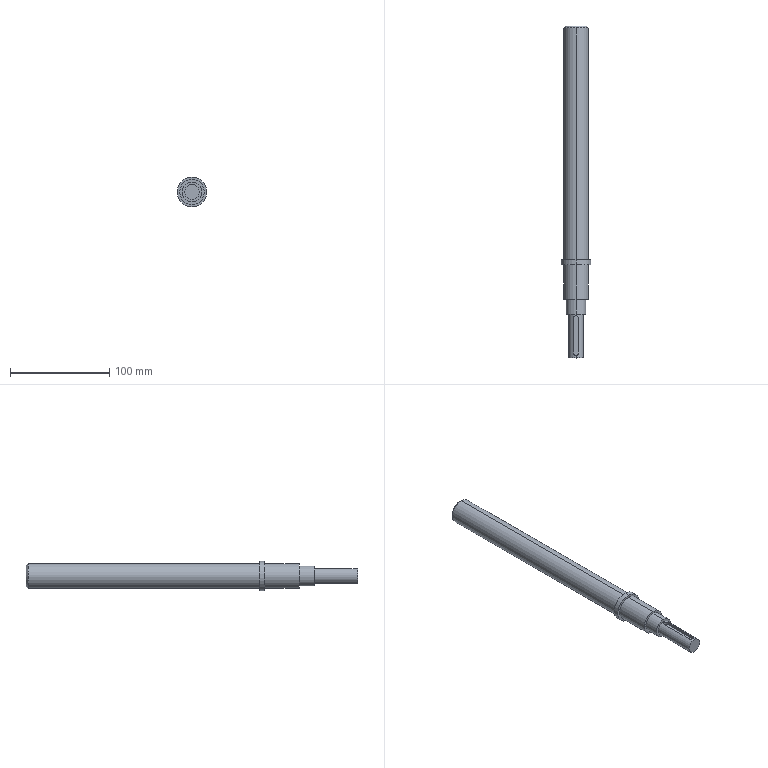Part | STEP file | MT-COMBO-119-S003 | 1 solid | 23 faces | box 30 x 334 x 30 mm | volume 147852 mm3 | cylinder 12 | plane 9 | cone 2 | commonest cylinder face diameters 25 x4 5 x2 15 x2 20 x2 30 x2
STEP:
#1=CARTESIAN_POINT('',(0.,334.,10.5));
#2=VERTEX_POINT('',#1);
#3=CARTESIAN_POINT('',(0.,334.,-10.5));
#4=VERTEX_POINT('',#3);
#5=CARTESIAN_POINT('',(0.,334.,0.));
#6=DIRECTION('',(0.,-1.,0.));
#7=DIRECTION('',(0.,0.,1.));
#8=AXIS2_PLACEMENT_3D('',#5,#6,#7);
#9=CIRCLE('',#8,10.5);
#10=EDGE_CURVE('',#2,#4,#9,.T.);
#11=ORIENTED_EDGE('',*,*,#10,.T.);
#12=CARTESIAN_POINT('',(0.,332.,-12.5));
#13=VERTEX_POINT('',#12);
#14=CARTESIAN_POINT('',(0.,334.,-10.5));
#15=DIRECTION('',(0.,-0.7071,-0.7071));
#16=VECTOR('',#15,1000.);
#17=LINE('',#14,#16);
#18=EDGE_CURVE('',#4,#13,#17,.T.);
#19=ORIENTED_EDGE('',*,*,#18,.T.);
#20=CARTESIAN_POINT('',(0.,332.,12.5));
#21=VERTEX_POINT('',#20);
#22=CARTESIAN_POINT('',(0.,332.,0.));
#23=DIRECTION('',(0.,1.,0.));
#24=DIRECTION('',(0.,0.,1.));
#25=AXIS2_PLACEMENT_3D('',#22,#23,#24);
#26=CIRCLE('',#25,12.5);
#27=EDGE_CURVE('',#13,#21,#26,.T.);
#28=ORIENTED_EDGE('',*,*,#27,.T.);
#29=CARTESIAN_POINT('',(0.,334.,10.5));
#30=DIRECTION('',(0.,-0.7071,0.7071));
#31=VECTOR('',#30,1000.);
#32=LINE('',#29,#31);
#33=EDGE_CURVE('',#2,#21,#32,.T.);
#34=ORIENTED_EDGE('',*,*,#33,.F.);
#35=EDGE_LOOP('',(#11,#19,#28,#34));
#36=FACE_OUTER_BOUND('',#35,.T.);
#37=CARTESIAN_POINT('',(0.,334.,0.));
#38=DIRECTION('',(0.,-1.,0.));
#39=DIRECTION('',(0.,0.,1.));
#40=AXIS2_PLACEMENT_3D('',#37,#38,#39);
#41=CONICAL_SURFACE('',#40,10.5,0.7854);
#42=ADVANCED_FACE('',(#36),#41,.T.);
#43=CARTESIAN_POINT('',(0.,99.,12.5));
#44=VERTEX_POINT('',#43);
#45=CARTESIAN_POINT('',(0.,99.,-12.5));
#46=VERTEX_POINT('',#45);
#47=CARTESIAN_POINT('',(0.,99.,0.));
#48=DIRECTION('',(0.,-1.,0.));
#49=DIRECTION('',(0.,0.,-1.));
#50=AXIS2_PLACEMENT_3D('',#47,#48,#49);
#51=CIRCLE('',#50,12.5);
#52=EDGE_CURVE('',#44,#46,#51,.T.);
#53=ORIENTED_EDGE('',*,*,#52,.F.);
#54=CARTESIAN_POINT('',(0.,334.,12.5));
#55=DIRECTION('',(0.,1.,0.));
#56=VECTOR('',#55,1000.);
#57=LINE('',#54,#56);
#58=EDGE_CURVE('',#44,#21,#57,.T.);
#59=ORIENTED_EDGE('',*,*,#58,.T.);
#60=ORIENTED_EDGE('',*,*,#27,.F.);
#61=CARTESIAN_POINT('',(0.,334.,-12.5));
#62=DIRECTION('',(0.,1.,0.));
#63=VECTOR('',#62,1000.);
#64=LINE('',#61,#63);
#65=EDGE_CURVE('',#46,#13,#64,.T.);
#66=ORIENTED_EDGE('',*,*,#65,.F.);
#67=EDGE_LOOP('',(#53,#59,#60,#66));
#68=FACE_OUTER_BOUND('',#67,.T.);
#69=CARTESIAN_POINT('',(0.,334.,0.));
#70=DIRECTION('',(0.,1.,0.));
#71=DIRECTION('',(0.,0.,-1.));
#72=AXIS2_PLACEMENT_3D('',#69,#70,#71);
#73=CYLINDRICAL_SURFACE('',#72,12.5);
#74=ADVANCED_FACE('',(#68),#73,.T.);
#75=CARTESIAN_POINT('',(0.,94.,15.));
#76=VERTEX_POINT('',#75);
#77=CARTESIAN_POINT('',(0.,94.,-15.));
#78=VERTEX_POINT('',#77);
#79=CARTESIAN_POINT('',(0.,94.,0.));
#80=DIRECTION('',(0.,-1.,0.));
#81=DIRECTION('',(0.,0.,-1.));
#82=AXIS2_PLACEMENT_3D('',#79,#80,#81);
#83=CIRCLE('',#82,15.);
#84=EDGE_CURVE('',#76,#78,#83,.T.);
#85=ORIENTED_EDGE('',*,*,#84,.F.);
#86=CARTESIAN_POINT('',(0.,99.,15.));
#87=VERTEX_POINT('',#86);
#88=CARTESIAN_POINT('',(0.,334.,15.));
#89=DIRECTION('',(0.,1.,0.));
#90=VECTOR('',#89,1000.);
#91=LINE('',#88,#90);
#92=EDGE_CURVE('',#76,#87,#91,.T.);
#93=ORIENTED_EDGE('',*,*,#92,.T.);
#94=CARTESIAN_POINT('',(0.,99.,-15.));
#95=VERTEX_POINT('',#94);
#96=CARTESIAN_POINT('',(0.,99.,0.));
#97=DIRECTION('',(0.,-1.,0.));
#98=DIRECTION('',(0.,0.,-1.));
#99=AXIS2_PLACEMENT_3D('',#96,#97,#98);
#100=CIRCLE('',#99,15.);
#101=EDGE_CURVE('',#87,#95,#100,.T.);
#102=ORIENTED_EDGE('',*,*,#101,.T.);
#103=CARTESIAN_POINT('',(0.,334.,-15.));
#104=DIRECTION('',(0.,1.,0.));
#105=VECTOR('',#104,1000.);
#106=LINE('',#103,#105);
#107=EDGE_CURVE('',#78,#95,#106,.T.);
#108=ORIENTED_EDGE('',*,*,#107,.F.);
#109=EDGE_LOOP('',(#85,#93,#102,#108));
#110=FACE_OUTER_BOUND('',#109,.T.);
#111=CARTESIAN_POINT('',(0.,334.,0.));
#112=DIRECTION('',(0.,1.,0.));
#113=DIRECTION('',(0.,0.,-1.));
#114=AXIS2_PLACEMENT_3D('',#111,#112,#113);
#115=CYLINDRICAL_SURFACE('',#114,15.);
#116=ADVANCED_FACE('',(#110),#115,.T.);
#117=CARTESIAN_POINT('',(0.,59.,12.5));
#118=VERTEX_POINT('',#117);
#119=CARTESIAN_POINT('',(0.,59.,-12.5));
#120=VERTEX_POINT('',#119);
#121=CARTESIAN_POINT('',(0.,59.,0.));
#122=DIRECTION('',(0.,-1.,0.));
#123=DIRECTION('',(0.,0.,-1.));
#124=AXIS2_PLACEMENT_3D('',#121,#122,#123);
#125=CIRCLE('',#124,12.5);
#126=EDGE_CURVE('',#118,#120,#125,.T.);
#127=ORIENTED_EDGE('',*,*,#126,.F.);
#128=CARTESIAN_POINT('',(0.,94.,12.5));
#129=VERTEX_POINT('',#128);
#130=CARTESIAN_POINT('',(0.,334.,12.5));
#131=DIRECTION('',(0.,1.,0.));
#132=VECTOR('',#131,1000.);
#133=LINE('',#130,#132);
#134=EDGE_CURVE('',#118,#129,#133,.T.);
#135=ORIENTED_EDGE('',*,*,#134,.T.);
#136=CARTESIAN_POINT('',(0.,94.,-12.5));
#137=VERTEX_POINT('',#136);
#138=CARTESIAN_POINT('',(0.,94.,0.));
#139=DIRECTION('',(0.,-1.,0.));
#140=DIRECTION('',(0.,0.,-1.));
#141=AXIS2_PLACEMENT_3D('',#138,#139,#140);
#142=CIRCLE('',#141,12.5);
#143=EDGE_CURVE('',#129,#137,#142,.T.);
#144=ORIENTED_EDGE('',*,*,#143,.T.);
#145=CARTESIAN_POINT('',(0.,334.,-12.5));
#146=DIRECTION('',(0.,1.,0.));
#147=VECTOR('',#146,1000.);
#148=LINE('',#145,#147);
#149=EDGE_CURVE('',#120,#137,#148,.T.);
#150=ORIENTED_EDGE('',*,*,#149,.F.);
#151=EDGE_LOOP('',(#127,#135,#144,#150));
#152=FACE_OUTER_BOUND('',#151,.T.);
#153=CARTESIAN_POINT('',(0.,334.,0.));
#154=DIRECTION('',(0.,1.,0.));
#155=DIRECTION('',(0.,0.,-1.));
#156=AXIS2_PLACEMENT_3D('',#153,#154,#155);
#157=CYLINDRICAL_SURFACE('',#156,12.5);
#158=ADVANCED_FACE('',(#152),#157,.T.);
#159=CARTESIAN_POINT('',(0.,44.,10.));
#160=VERTEX_POINT('',#159);
#161=CARTESIAN_POINT('',(0.,44.,-10.));
#162=VERTEX_POINT('',#161);
#163=CARTESIAN_POINT('',(0.,44.,0.));
#164=DIRECTION('',(0.,-1.,0.));
#165=DIRECTION('',(0.,0.,-1.));
#166=AXIS2_PLACEMENT_3D('',#163,#164,#165);
#167=CIRCLE('',#166,10.);
#168=EDGE_CURVE('',#160,#162,#167,.T.);
#169=ORIENTED_EDGE('',*,*,#168,.F.);
#170=CARTESIAN_POINT('',(0.,59.,10.));
#171=VERTEX_POINT('',#170);
#172=CARTESIAN_POINT('',(0.,334.,10.));
#173=DIRECTION('',(0.,1.,0.));
#174=VECTOR('',#173,1000.);
#175=LINE('',#172,#174);
#176=EDGE_CURVE('',#160,#171,#175,.T.);
#177=ORIENTED_EDGE('',*,*,#176,.T.);
#178=CARTESIAN_POINT('',(0.,59.,-10.));
#179=VERTEX_POINT('',#178);
#180=CARTESIAN_POINT('',(0.,59.,0.));
#181=DIRECTION('',(0.,-1.,0.));
#182=DIRECTION('',(0.,0.,-1.));
#183=AXIS2_PLACEMENT_3D('',#180,#181,#182);
#184=CIRCLE('',#183,10.);
#185=EDGE_CURVE('',#171,#179,#184,.T.);
#186=ORIENTED_EDGE('',*,*,#185,.T.);
#187=CARTESIAN_POINT('',(0.,334.,-10.));
#188=DIRECTION('',(0.,1.,0.));
#189=VECTOR('',#188,1000.);
#190=LINE('',#187,#189);
#191=EDGE_CURVE('',#162,#179,#190,.T.);
#192=ORIENTED_EDGE('',*,*,#191,.F.);
#193=EDGE_LOOP('',(#169,#177,#186,#192));
#194=FACE_OUTER_BOUND('',#193,.T.);
#195=CARTESIAN_POINT('',(0.,334.,0.));
#196=DIRECTION('',(0.,1.,0.));
#197=DIRECTION('',(0.,0.,-1.));
#198=AXIS2_PLACEMENT_3D('',#195,#196,#197);
#199=CYLINDRICAL_SURFACE('',#198,10.);
#200=ADVANCED_FACE('',(#194),#199,.T.);
#201=CARTESIAN_POINT('',(0.,0.,7.5));
#202=VERTEX_POINT('',#201);
#203=CARTESIAN_POINT('',(0.,0.,-7.5));
#204=VERTEX_POINT('',#203);
#205=CARTESIAN_POINT('',(0.,0.,0.));
#206=DIRECTION('',(0.,-1.,0.));
#207=DIRECTION('',(0.,0.,-1.));
#208=AXIS2_PLACEMENT_3D('',#205,#206,#207);
#209=CIRCLE('',#208,7.5);
#210=EDGE_CURVE('',#202,#204,#209,.T.);
#211=ORIENTED_EDGE('',*,*,#210,.F.);
#212=CARTESIAN_POINT('',(0.,2.5,7.5));
#213=VERTEX_POINT('',#212);
#214=CARTESIAN_POINT('',(0.,334.,7.5));
#215=DIRECTION('',(0.,1.,0.));
#216=VECTOR('',#215,1000.);
#217=LINE('',#214,#216);
#218=EDGE_CURVE('',#202,#213,#217,.T.);
#219=ORIENTED_EDGE('',*,*,#218,.T.);
#220=CARTESIAN_POINT('',(-2.5,5.,7.071));
#221=VERTEX_POINT('',#220);
#222=CARTESIAN_POINT('',(-2.5,5.,7.071));
#223=CARTESIAN_POINT('',(-2.5,4.833,7.071));
#224=CARTESIAN_POINT('',(-2.484,4.67,7.077));
#225=CARTESIAN_POINT('',(-2.419,4.349,7.099));
#226=CARTESIAN_POINT('',(-2.371,4.189,7.116));
#227=CARTESIAN_POINT('',(-2.245,3.887,7.157));
#228=CARTESIAN_POINT('',(-2.168,3.744,7.181));
#229=CARTESIAN_POINT('',(-1.986,3.473,7.233));
#230=CARTESIAN_POINT('',(-1.882,3.346,7.261));
#231=CARTESIAN_POINT('',(-1.538,3.003,7.344));
#232=CARTESIAN_POINT('',(-1.261,2.817,7.399));
#233=CARTESIAN_POINT('',(-0.81,2.629,7.458));
#234=CARTESIAN_POINT('',(-0.6511,2.581,7.473));
#235=CARTESIAN_POINT('',(-0.3276,2.516,7.495));
#236=CARTESIAN_POINT('',(-0.1645,2.5,7.5));
#237=CARTESIAN_POINT('',(0.,2.5,7.5));
#238=B_SPLINE_CURVE_WITH_KNOTS('',3,(#222,#223,#224,#225,#226,#227,#228,#229,#230,#231,#232,#233,#234,#235,#236,#237),.UNSPECIFIED.,.F.,.F.,(4,2,2,2,2,2,2,4),(0.,0.0004922,0.0009844,0.001477,0.001969,0.002953,0.003445,0.003937),.UNSPECIFIED.);
#239=EDGE_CURVE('',#221,#213,#238,.T.);
#240=ORIENTED_EDGE('',*,*,#239,.F.);
#241=CARTESIAN_POINT('',(-2.5,40.,7.071));
#242=VERTEX_POINT('',#241);
#243=CARTESIAN_POINT('',(-2.5,334.,7.071));
#244=DIRECTION('',(0.,-1.,0.));
#245=VECTOR('',#244,1000.);
#246=LINE('',#243,#245);
#247=EDGE_CURVE('',#242,#221,#246,.T.);
#248=ORIENTED_EDGE('',*,*,#247,.F.);
#249=CARTESIAN_POINT('',(0.,42.5,7.5));
#250=VERTEX_POINT('',#249);
#251=CARTESIAN_POINT('',(0.,42.5,7.5));
#252=CARTESIAN_POINT('',(-0.1643,42.5,7.5));
#253=CARTESIAN_POINT('',(-0.3311,42.483,7.494));
#254=CARTESIAN_POINT('',(-0.6524,42.419,7.473));
#255=CARTESIAN_POINT('',(-0.8088,42.371,7.458));
#256=CARTESIAN_POINT('',(-1.113,42.245,7.419));
#257=CARTESIAN_POINT('',(-1.257,42.167,7.395));
#258=CARTESIAN_POINT('',(-1.526,41.987,7.344));
#259=CARTESIAN_POINT('',(-1.653,41.882,7.316));
#260=CARTESIAN_POINT('',(-1.883,41.652,7.261));
#261=CARTESIAN_POINT('',(-1.986,41.527,7.233));
#262=CARTESIAN_POINT('',(-2.167,41.258,7.181));
#263=CARTESIAN_POINT('',(-2.245,41.112,7.156));
#264=CARTESIAN_POINT('',(-2.37,40.811,7.116));
#265=CARTESIAN_POINT('',(-2.418,40.656,7.1));
#266=CARTESIAN_POINT('',(-2.483,40.332,7.077));
#267=CARTESIAN_POINT('',(-2.5,40.166,7.071));
#268=CARTESIAN_POINT('',(-2.5,40.,7.071));
#269=B_SPLINE_CURVE_WITH_KNOTS('',3,(#251,#252,#253,#254,#255,#256,#257,#258,#259,#260,#261,#262,#263,#264,#265,#266,#267,#268),.UNSPECIFIED.,.F.,.F.,(4,2,2,2,2,2,2,2,4),(0.003937,0.004429,0.004921,0.005412,0.005904,0.006395,0.006887,0.007378,0.00787),.UNSPECIFIED.);
#270=EDGE_CURVE('',#250,#242,#269,.T.);
#271=ORIENTED_EDGE('',*,*,#270,.F.);
#272=CARTESIAN_POINT('',(0.,44.,7.5));
#273=VERTEX_POINT('',#272);
#274=CARTESIAN_POINT('',(0.,334.,7.5));
#275=DIRECTION('',(0.,1.,0.));
#276=VECTOR('',#275,1000.);
#277=LINE('',#274,#276);
#278=EDGE_CURVE('',#250,#273,#277,.T.);
#279=ORIENTED_EDGE('',*,*,#278,.T.);
#280=CARTESIAN_POINT('',(0.,44.,-7.5));
#281=VERTEX_POINT('',#280);
#282=CARTESIAN_POINT('',(0.,44.,0.));
#283=DIRECTION('',(0.,-1.,0.));
#284=DIRECTION('',(0.,0.,-1.));
#285=AXIS2_PLACEMENT_3D('',#282,#283,#284);
#286=CIRCLE('',#285,7.5);
#287=EDGE_CURVE('',#273,#281,#286,.T.);
#288=ORIENTED_EDGE('',*,*,#287,.T.);
#289=CARTESIAN_POINT('',(0.,334.,-7.5));
#290=DIRECTION('',(0.,1.,0.));
#291=VECTOR('',#290,1000.);
#292=LINE('',#289,#291);
#293=EDGE_CURVE('',#204,#281,#292,.T.);
#294=ORIENTED_EDGE('',*,*,#293,.F.);
#295=EDGE_LOOP('',(#211,#219,#240,#248,#271,#279,#288,#294));
#296=FACE_OUTER_BOUND('',#295,.T.);
#297=CARTESIAN_POINT('',(0.,334.,0.));
#298=DIRECTION('',(0.,1.,0.));
#299=DIRECTION('',(0.,0.,-1.));
#300=AXIS2_PLACEMENT_3D('',#297,#298,#299);
#301=CYLINDRICAL_SURFACE('',#300,7.5);
#302=ADVANCED_FACE('',(#296),#301,.T.);
#303=CARTESIAN_POINT('',(0.,0.,0.));
#304=DIRECTION('',(0.,-1.,0.));
#305=DIRECTION('',(0.,0.,-1.));
#306=AXIS2_PLACEMENT_3D('',#303,#304,#305);
#307=CIRCLE('',#306,7.5);
#308=EDGE_CURVE('',#204,#202,#307,.T.);
#309=ORIENTED_EDGE('',*,*,#308,.T.);
#310=ORIENTED_EDGE('',*,*,#210,.T.);
#311=EDGE_LOOP('',(#309,#310));
#312=FACE_OUTER_BOUND('',#311,.T.);
#313=CARTESIAN_POINT('',(0.,0.,0.));
#314=DIRECTION('',(0.,1.,0.));
#315=DIRECTION('',(0.,0.,-1.));
#316=AXIS2_PLACEMENT_3D('',#313,#314,#315);
#317=PLANE('',#316);
#318=ADVANCED_FACE('',(#312),#317,.F.);
#319=ORIENTED_EDGE('',*,*,#218,.F.);
#320=ORIENTED_EDGE('',*,*,#308,.F.);
#321=ORIENTED_EDGE('',*,*,#293,.T.);
#322=CARTESIAN_POINT('',(0.,44.,0.));
#323=DIRECTION('',(0.,-1.,0.));
#324=DIRECTION('',(0.,0.,-1.));
#325=AXIS2_PLACEMENT_3D('',#322,#323,#324);
#326=CIRCLE('',#325,7.5);
#327=EDGE_CURVE('',#281,#273,#326,.T.);
#328=ORIENTED_EDGE('',*,*,#327,.T.);
#329=ORIENTED_EDGE('',*,*,#278,.F.);
#330=CARTESIAN_POINT('',(2.5,40.,7.071));
#331=VERTEX_POINT('',#330);
#332=CARTESIAN_POINT('',(2.5,40.,7.071));
#333=CARTESIAN_POINT('',(2.5,40.167,7.071));
#334=CARTESIAN_POINT('',(2.484,40.33,7.077));
#335=CARTESIAN_POINT('',(2.419,40.651,7.099));
#336=CARTESIAN_POINT('',(2.371,40.811,7.116));
#337=CARTESIAN_POINT('',(2.245,41.113,7.157));
#338=CARTESIAN_POINT('',(2.168,41.256,7.181));
#339=CARTESIAN_POINT('',(1.986,41.527,7.233));
#340=CARTESIAN_POINT('',(1.882,41.654,7.261));
#341=CARTESIAN_POINT('',(1.538,41.997,7.344));
#342=CARTESIAN_POINT('',(1.261,42.183,7.399));
#343=CARTESIAN_POINT('',(0.81,42.371,7.458));
#344=CARTESIAN_POINT('',(0.6511,42.419,7.473));
#345=CARTESIAN_POINT('',(0.3276,42.484,7.495));
#346=CARTESIAN_POINT('',(0.1645,42.5,7.5));
#347=CARTESIAN_POINT('',(0.,42.5,7.5));
#348=B_SPLINE_CURVE_WITH_KNOTS('',3,(#332,#333,#334,#335,#336,#337,#338,#339,#340,#341,#342,#343,#344,#345,#346,#347),.UNSPECIFIED.,.F.,.F.,(4,2,2,2,2,2,2,4),(0.,0.0004922,0.0009844,0.001477,0.001969,0.002953,0.003445,0.003937),.UNSPECIFIED.);
#349=EDGE_CURVE('',#331,#250,#348,.T.);
#350=ORIENTED_EDGE('',*,*,#349,.F.);
#351=CARTESIAN_POINT('',(2.5,5.,7.071));
#352=VERTEX_POINT('',#351);
#353=CARTESIAN_POINT('',(2.5,334.,7.071));
#354=DIRECTION('',(0.,1.,0.));
#355=VECTOR('',#354,1000.);
#356=LINE('',#353,#355);
#357=EDGE_CURVE('',#352,#331,#356,.T.);
#358=ORIENTED_EDGE('',*,*,#357,.F.);
#359=CARTESIAN_POINT('',(0.,2.5,7.5));
#360=CARTESIAN_POINT('',(0.1643,2.5,7.5));
#361=CARTESIAN_POINT('',(0.3311,2.517,7.494));
#362=CARTESIAN_POINT('',(0.6524,2.581,7.473));
#363=CARTESIAN_POINT('',(0.8088,2.629,7.458));
#364=CARTESIAN_POINT('',(1.113,2.755,7.419));
#365=CARTESIAN_POINT('',(1.257,2.833,7.395));
#366=CARTESIAN_POINT('',(1.526,3.013,7.344));
#367=CARTESIAN_POINT('',(1.653,3.118,7.316));
#368=CARTESIAN_POINT('',(1.883,3.348,7.261));
#369=CARTESIAN_POINT('',(1.986,3.473,7.233));
#370=CARTESIAN_POINT('',(2.167,3.742,7.181));
#371=CARTESIAN_POINT('',(2.245,3.888,7.156));
#372=CARTESIAN_POINT('',(2.37,4.189,7.116));
#373=CARTESIAN_POINT('',(2.418,4.344,7.1));
#374=CARTESIAN_POINT('',(2.483,4.668,7.077));
#375=CARTESIAN_POINT('',(2.5,4.834,7.071));
#376=CARTESIAN_POINT('',(2.5,5.,7.071));
#377=B_SPLINE_CURVE_WITH_KNOTS('',3,(#359,#360,#361,#362,#363,#364,#365,#366,#367,#368,#369,#370,#371,#372,#373,#374,#375,#376),.UNSPECIFIED.,.F.,.F.,(4,2,2,2,2,2,2,2,4),(0.003937,0.004429,0.004921,0.005412,0.005904,0.006395,0.006887,0.007378,0.00787),.UNSPECIFIED.);
#378=EDGE_CURVE('',#213,#352,#377,.T.);
#379=ORIENTED_EDGE('',*,*,#378,.F.);
#380=EDGE_LOOP('',(#319,#320,#321,#328,#329,#350,#358,#379));
#381=FACE_OUTER_BOUND('',#380,.T.);
#382=CARTESIAN_POINT('',(0.,334.,0.));
#383=DIRECTION('',(0.,1.,0.));
#384=DIRECTION('',(0.,0.,-1.));
#385=AXIS2_PLACEMENT_3D('',#382,#383,#384);
#386=CYLINDRICAL_SURFACE('',#385,7.5);
#387=ADVANCED_FACE('',(#381),#386,.T.);
#388=CARTESIAN_POINT('',(0.,44.,0.));
#389=DIRECTION('',(0.,-1.,0.));
#390=DIRECTION('',(0.,0.,-1.));
#391=AXIS2_PLACEMENT_3D('',#388,#389,#390);
#392=CIRCLE('',#391,10.);
#393=EDGE_CURVE('',#162,#160,#392,.T.);
#394=ORIENTED_EDGE('',*,*,#393,.T.);
#395=ORIENTED_EDGE('',*,*,#168,.T.);
#396=EDGE_LOOP('',(#394,#395));
#397=FACE_OUTER_BOUND('',#396,.T.);
#398=ORIENTED_EDGE('',*,*,#327,.F.);
#399=ORIENTED_EDGE('',*,*,#287,.F.);
#400=EDGE_LOOP('',(#398,#399));
#401=FACE_BOUND('',#400,.T.);
#402=CARTESIAN_POINT('',(0.,44.,7.5));
#403=DIRECTION('',(0.,1.,0.));
#404=DIRECTION('',(0.,0.,-1.));
#405=AXIS2_PLACEMENT_3D('',#402,#403,#404);
#406=PLANE('',#405);
#407=ADVANCED_FACE('',(#397,#401),#406,.F.);
#408=ORIENTED_EDGE('',*,*,#176,.F.);
#409=ORIENTED_EDGE('',*,*,#393,.F.);
#410=ORIENTED_EDGE('',*,*,#191,.T.);
#411=CARTESIAN_POINT('',(0.,59.,0.));
#412=DIRECTION('',(0.,-1.,0.));
#413=DIRECTION('',(0.,0.,-1.));
#414=AXIS2_PLACEMENT_3D('',#411,#412,#413);
#415=CIRCLE('',#414,10.);
#416=EDGE_CURVE('',#179,#171,#415,.T.);
#417=ORIENTED_EDGE('',*,*,#416,.T.);
#418=EDGE_LOOP('',(#408,#409,#410,#417));
#419=FACE_OUTER_BOUND('',#418,.T.);
#420=CARTESIAN_POINT('',(0.,334.,0.));
#421=DIRECTION('',(0.,1.,0.));
#422=DIRECTION('',(0.,0.,-1.));
#423=AXIS2_PLACEMENT_3D('',#420,#421,#422);
#424=CYLINDRICAL_SURFACE('',#423,10.);
#425=ADVANCED_FACE('',(#419),#424,.T.);
#426=CARTESIAN_POINT('',(0.,59.,0.));
#427=DIRECTION('',(0.,-1.,0.));
#428=DIRECTION('',(0.,0.,-1.));
#429=AXIS2_PLACEMENT_3D('',#426,#427,#428);
#430=CIRCLE('',#429,12.5);
#431=EDGE_CURVE('',#120,#118,#430,.T.);
#432=ORIENTED_EDGE('',*,*,#431,.T.);
#433=ORIENTED_EDGE('',*,*,#126,.T.);
#434=EDGE_LOOP('',(#432,#433));
#435=FACE_OUTER_BOUND('',#434,.T.);
#436=ORIENTED_EDGE('',*,*,#416,.F.);
#437=ORIENTED_EDGE('',*,*,#185,.F.);
#438=EDGE_LOOP('',(#436,#437));
#439=FACE_BOUND('',#438,.T.);
#440=CARTESIAN_POINT('',(0.,59.,10.));
#441=DIRECTION('',(0.,1.,0.));
#442=DIRECTION('',(0.,0.,-1.));
#443=AXIS2_PLACEMENT_3D('',#440,#441,#442);
#444=PLANE('',#443);
#445=ADVANCED_FACE('',(#435,#439),#444,.F.);
#446=ORIENTED_EDGE('',*,*,#134,.F.);
#447=ORIENTED_EDGE('',*,*,#431,.F.);
#448=ORIENTED_EDGE('',*,*,#149,.T.);
#449=CARTESIAN_POINT('',(0.,94.,0.));
#450=DIRECTION('',(0.,-1.,0.));
#451=DIRECTION('',(0.,0.,-1.));
#452=AXIS2_PLACEMENT_3D('',#449,#450,#451);
#453=CIRCLE('',#452,12.5);
#454=EDGE_CURVE('',#137,#129,#453,.T.);
#455=ORIENTED_EDGE('',*,*,#454,.T.);
#456=EDGE_LOOP('',(#446,#447,#448,#455));
#457=FACE_OUTER_BOUND('',#456,.T.);
#458=CARTESIAN_POINT('',(0.,334.,0.));
#459=DIRECTION('',(0.,1.,0.));
#460=DIRECTION('',(0.,0.,-1.));
#461=AXIS2_PLACEMENT_3D('',#458,#459,#460);
#462=CYLINDRICAL_SURFACE('',#461,12.5);
#463=ADVANCED_FACE('',(#457),#462,.T.);
#464=CARTESIAN_POINT('',(0.,94.,0.));
#465=DIRECTION('',(0.,-1.,0.));
#466=DIRECTION('',(0.,0.,-1.));
#467=AXIS2_PLACEMENT_3D('',#464,#465,#466);
#468=CIRCLE('',#467,15.);
#469=EDGE_CURVE('',#78,#76,#468,.T.);
#470=ORIENTED_EDGE('',*,*,#469,.T.);
#471=ORIENTED_EDGE('',*,*,#84,.T.);
#472=EDGE_LOOP('',(#470,#471));
#473=FACE_OUTER_BOUND('',#472,.T.);
#474=ORIENTED_EDGE('',*,*,#454,.F.);
#475=ORIENTED_EDGE('',*,*,#143,.F.);
#476=EDGE_LOOP('',(#474,#475));
#477=FACE_BOUND('',#476,.T.);
#478=CARTESIAN_POINT('',(0.,94.,12.5));
#479=DIRECTION('',(0.,1.,0.));
#480=DIRECTION('',(0.,0.,-1.));
#481=AXIS2_PLACEMENT_3D('',#478,#479,#480);
#482=PLANE('',#481);
#483=ADVANCED_FACE('',(#473,#477),#482,.F.);
#484=ORIENTED_EDGE('',*,*,#92,.F.);
#485=ORIENTED_EDGE('',*,*,#469,.F.);
#486=ORIENTED_EDGE('',*,*,#107,.T.);
#487=CARTESIAN_POINT('',(0.,99.,0.));
#488=DIRECTION('',(0.,-1.,0.));
#489=DIRECTION('',(0.,0.,-1.));
#490=AXIS2_PLACEMENT_3D('',#487,#488,#489);
#491=CIRCLE('',#490,15.);
#492=EDGE_CURVE('',#95,#87,#491,.T.);
#493=ORIENTED_EDGE('',*,*,#492,.T.);
#494=EDGE_LOOP('',(#484,#485,#486,#493));
#495=FACE_OUTER_BOUND('',#494,.T.);
#496=CARTESIAN_POINT('',(0.,334.,0.));
#497=DIRECTION('',(0.,1.,0.));
#498=DIRECTION('',(0.,0.,-1.));
#499=AXIS2_PLACEMENT_3D('',#496,#497,#498);
#500=CYLINDRICAL_SURFACE('',#499,15.);
#501=ADVANCED_FACE('',(#495),#500,.T.);
#502=CARTESIAN_POINT('',(0.,99.,0.));
#503=DIRECTION('',(0.,-1.,0.));
#504=DIRECTION('',(0.,0.,-1.));
#505=AXIS2_PLACEMENT_3D('',#502,#503,#504);
#506=CIRCLE('',#505,12.5);
#507=EDGE_CURVE('',#46,#44,#506,.T.);
#508=ORIENTED_EDGE('',*,*,#507,.T.);
#509=ORIENTED_EDGE('',*,*,#52,.T.);
#510=EDGE_LOOP('',(#508,#509));
#511=FACE_BOUND('',#510,.T.);
#512=ORIENTED_EDGE('',*,*,#492,.F.);
#513=ORIENTED_EDGE('',*,*,#101,.F.);
#514=EDGE_LOOP('',(#512,#513));
#515=FACE_OUTER_BOUND('',#514,.T.);
#516=CARTESIAN_POINT('',(0.,99.,15.));
#517=DIRECTION('',(0.,-1.,0.));
#518=DIRECTION('',(0.,0.,1.));
#519=AXIS2_PLACEMENT_3D('',#516,#517,#518);
#520=PLANE('',#519);
#521=ADVANCED_FACE('',(#511,#515),#520,.F.);
#522=ORIENTED_EDGE('',*,*,#58,.F.);
#523=ORIENTED_EDGE('',*,*,#507,.F.);
#524=ORIENTED_EDGE('',*,*,#65,.T.);
#525=CARTESIAN_POINT('',(0.,332.,0.));
#526=DIRECTION('',(0.,1.,0.));
#527=DIRECTION('',(0.,0.,1.));
#528=AXIS2_PLACEMENT_3D('',#525,#526,#527);
#529=CIRCLE('',#528,12.5);
#530=EDGE_CURVE('',#21,#13,#529,.T.);
#531=ORIENTED_EDGE('',*,*,#530,.F.);
#532=EDGE_LOOP('',(#522,#523,#524,#531));
#533=FACE_OUTER_BOUND('',#532,.T.);
#534=CARTESIAN_POINT('',(0.,334.,0.));
#535=DIRECTION('',(0.,1.,0.));
#536=DIRECTION('',(0.,0.,-1.));
#537=AXIS2_PLACEMENT_3D('',#534,#535,#536);
#538=CYLINDRICAL_SURFACE('',#537,12.5);
#539=ADVANCED_FACE('',(#533),#538,.T.);
#540=ORIENTED_EDGE('',*,*,#10,.F.);
#541=CARTESIAN_POINT('',(0.,334.,0.));
#542=DIRECTION('',(0.,-1.,0.));
#543=DIRECTION('',(0.,0.,1.));
#544=AXIS2_PLACEMENT_3D('',#541,#542,#543);
#545=CIRCLE('',#544,10.5);
#546=EDGE_CURVE('',#4,#2,#545,.T.);
#547=ORIENTED_EDGE('',*,*,#546,.F.);
#548=EDGE_LOOP('',(#540,#547));
#549=FACE_OUTER_BOUND('',#548,.T.);
#550=CARTESIAN_POINT('',(0.,334.,0.));
#551=DIRECTION('',(0.,-1.,0.));
#552=DIRECTION('',(0.,0.,1.));
#553=AXIS2_PLACEMENT_3D('',#550,#551,#552);
#554=PLANE('',#553);
#555=ADVANCED_FACE('',(#549),#554,.F.);
#556=ORIENTED_EDGE('',*,*,#18,.F.);
#557=ORIENTED_EDGE('',*,*,#546,.T.);
#558=ORIENTED_EDGE('',*,*,#33,.T.);
#559=ORIENTED_EDGE('',*,*,#530,.T.);
#560=EDGE_LOOP('',(#556,#557,#558,#559));
#561=FACE_OUTER_BOUND('',#560,.T.);
#562=CARTESIAN_POINT('',(0.,334.,0.));
#563=DIRECTION('',(0.,-1.,0.));
#564=DIRECTION('',(0.,0.,1.));
#565=AXIS2_PLACEMENT_3D('',#562,#563,#564);
#566=CONICAL_SURFACE('',#565,10.5,0.7854);
#567=ADVANCED_FACE('',(#561),#566,.T.);
#568=CARTESIAN_POINT('',(2.5,40.,4.5));
#569=VERTEX_POINT('',#568);
#570=CARTESIAN_POINT('',(2.5,40.,15.));
#571=DIRECTION('',(0.,0.,-1.));
#572=VECTOR('',#571,1000.);
#573=LINE('',#570,#572);
#574=EDGE_CURVE('',#331,#569,#573,.T.);
#575=ORIENTED_EDGE('',*,*,#574,.F.);
#576=ORIENTED_EDGE('',*,*,#349,.T.);
#577=ORIENTED_EDGE('',*,*,#270,.T.);
#578=CARTESIAN_POINT('',(-2.5,40.,4.5));
#579=VERTEX_POINT('',#578);
#580=CARTESIAN_POINT('',(-2.5,40.,15.));
#581=DIRECTION('',(0.,0.,-1.));
#582=VECTOR('',#581,1000.);
#583=LINE('',#580,#582);
#584=EDGE_CURVE('',#242,#579,#583,.T.);
#585=ORIENTED_EDGE('',*,*,#584,.T.);
#586=CARTESIAN_POINT('',(0.,40.,4.5));
#587=DIRECTION('',(0.,0.,1.));
#588=DIRECTION('',(1.,0.,0.));
#589=AXIS2_PLACEMENT_3D('',#586,#587,#588);
#590=CIRCLE('',#589,2.5);
#591=EDGE_CURVE('',#569,#579,#590,.T.);
#592=ORIENTED_EDGE('',*,*,#591,.F.);
#593=EDGE_LOOP('',(#575,#576,#577,#585,#592));
#594=FACE_OUTER_BOUND('',#593,.T.);
#595=CARTESIAN_POINT('',(0.,40.,15.));
#596=DIRECTION('',(0.,0.,-1.));
#597=DIRECTION('',(1.,0.,0.));
#598=AXIS2_PLACEMENT_3D('',#595,#596,#597);
#599=CYLINDRICAL_SURFACE('',#598,2.5);
#600=ADVANCED_FACE('',(#594),#599,.F.);
#601=CARTESIAN_POINT('',(2.5,5.,4.5));
#602=VERTEX_POINT('',#601);
#603=CARTESIAN_POINT('',(2.5,5.,15.));
#604=DIRECTION('',(0.,0.,-1.));
#605=VECTOR('',#604,1000.);
#606=LINE('',#603,#605);
#607=EDGE_CURVE('',#352,#602,#606,.T.);
#608=ORIENTED_EDGE('',*,*,#607,.F.);
#609=ORIENTED_EDGE('',*,*,#357,.T.);
#610=ORIENTED_EDGE('',*,*,#574,.T.);
#611=CARTESIAN_POINT('',(2.5,40.,4.5));
#612=DIRECTION('',(0.,1.,0.));
#613=VECTOR('',#612,1000.);
#614=LINE('',#611,#613);
#615=EDGE_CURVE('',#602,#569,#614,.T.);
#616=ORIENTED_EDGE('',*,*,#615,.F.);
#617=EDGE_LOOP('',(#608,#609,#610,#616));
#618=FACE_OUTER_BOUND('',#617,.T.);
#619=CARTESIAN_POINT('',(2.5,40.,15.));
#620=DIRECTION('',(1.,0.,0.));
#621=DIRECTION('',(0.,1.,0.));
#622=AXIS2_PLACEMENT_3D('',#619,#620,#621);
#623=PLANE('',#622);
#624=ADVANCED_FACE('',(#618),#623,.F.);
#625=CARTESIAN_POINT('',(-2.5,5.,4.5));
#626=VERTEX_POINT('',#625);
#627=CARTESIAN_POINT('',(-2.5,5.,15.));
#628=DIRECTION('',(0.,0.,-1.));
#629=VECTOR('',#628,1000.);
#630=LINE('',#627,#629);
#631=EDGE_CURVE('',#221,#626,#630,.T.);
#632=ORIENTED_EDGE('',*,*,#631,.F.);
#633=ORIENTED_EDGE('',*,*,#239,.T.);
#634=ORIENTED_EDGE('',*,*,#378,.T.);
#635=ORIENTED_EDGE('',*,*,#607,.T.);
#636=CARTESIAN_POINT('',(0.,5.,4.5));
#637=DIRECTION('',(0.,0.,1.));
#638=DIRECTION('',(1.,0.,0.));
#639=AXIS2_PLACEMENT_3D('',#636,#637,#638);
#640=CIRCLE('',#639,2.5);
#641=EDGE_CURVE('',#626,#602,#640,.T.);
#642=ORIENTED_EDGE('',*,*,#641,.F.);
#643=EDGE_LOOP('',(#632,#633,#634,#635,#642));
#644=FACE_OUTER_BOUND('',#643,.T.);
#645=CARTESIAN_POINT('',(0.,5.,15.));
#646=DIRECTION('',(0.,0.,-1.));
#647=DIRECTION('',(1.,0.,0.));
#648=AXIS2_PLACEMENT_3D('',#645,#646,#647);
#649=CYLINDRICAL_SURFACE('',#648,2.5);
#650=ADVANCED_FACE('',(#644),#649,.F.);
#651=ORIENTED_EDGE('',*,*,#584,.F.);
#652=ORIENTED_EDGE('',*,*,#247,.T.);
#653=ORIENTED_EDGE('',*,*,#631,.T.);
#654=CARTESIAN_POINT('',(-2.5,40.,4.5));
#655=DIRECTION('',(0.,-1.,0.));
#656=VECTOR('',#655,1000.);
#657=LINE('',#654,#656);
#658=EDGE_CURVE('',#579,#626,#657,.T.);
#659=ORIENTED_EDGE('',*,*,#658,.F.);
#660=EDGE_LOOP('',(#651,#652,#653,#659));
#661=FACE_OUTER_BOUND('',#660,.T.);
#662=CARTESIAN_POINT('',(-2.5,40.,15.));
#663=DIRECTION('',(-1.,0.,0.));
#664=DIRECTION('',(0.,-1.,0.));
#665=AXIS2_PLACEMENT_3D('',#662,#663,#664);
#666=PLANE('',#665);
#667=ADVANCED_FACE('',(#661),#666,.F.);
#668=ORIENTED_EDGE('',*,*,#591,.T.);
#669=ORIENTED_EDGE('',*,*,#658,.T.);
#670=ORIENTED_EDGE('',*,*,#641,.T.);
#671=ORIENTED_EDGE('',*,*,#615,.T.);
#672=EDGE_LOOP('',(#668,#669,#670,#671));
#673=FACE_OUTER_BOUND('',#672,.T.);
#674=CARTESIAN_POINT('',(0.,40.,4.5));
#675=DIRECTION('',(0.,0.,-1.));
#676=DIRECTION('',(1.,0.,0.));
#677=AXIS2_PLACEMENT_3D('',#674,#675,#676);
#678=PLANE('',#677);
#679=ADVANCED_FACE('',(#673),#678,.F.);
#680=CLOSED_SHELL('',(#42,#74,#116,#158,#200,#302,#318,#387,#407,#425,#445,#463,#483,#501,#521,#539,#555,#567,#600,#624,#650,#667,#679));
#681=MANIFOLD_SOLID_BREP('',#680);
#682=CARTESIAN_POINT('',(0.,0.,0.));
#683=DIRECTION('',(0.,0.,1.));
#684=DIRECTION('',(1.,0.,0.));
#685=AXIS2_PLACEMENT_3D('',#682,#683,#684);
#686=(LENGTH_UNIT()NAMED_UNIT(*)SI_UNIT(.MILLI.,.METRE.));
#687=UNCERTAINTY_MEASURE_WITH_UNIT(LENGTH_MEASURE(0.00001),#686,'','');
#688=(NAMED_UNIT(*)PLANE_ANGLE_UNIT()SI_UNIT($,.RADIAN.));
#689=(NAMED_UNIT(*)SI_UNIT($,.STERADIAN.)SOLID_ANGLE_UNIT());
#690=(GEOMETRIC_REPRESENTATION_CONTEXT(3)GLOBAL_UNCERTAINTY_ASSIGNED_CONTEXT((#687))GLOBAL_UNIT_ASSIGNED_CONTEXT((#686,#688,#689))REPRESENTATION_CONTEXT('',''));
#691=ADVANCED_BREP_SHAPE_REPRESENTATION('',(#681,#685),#690);